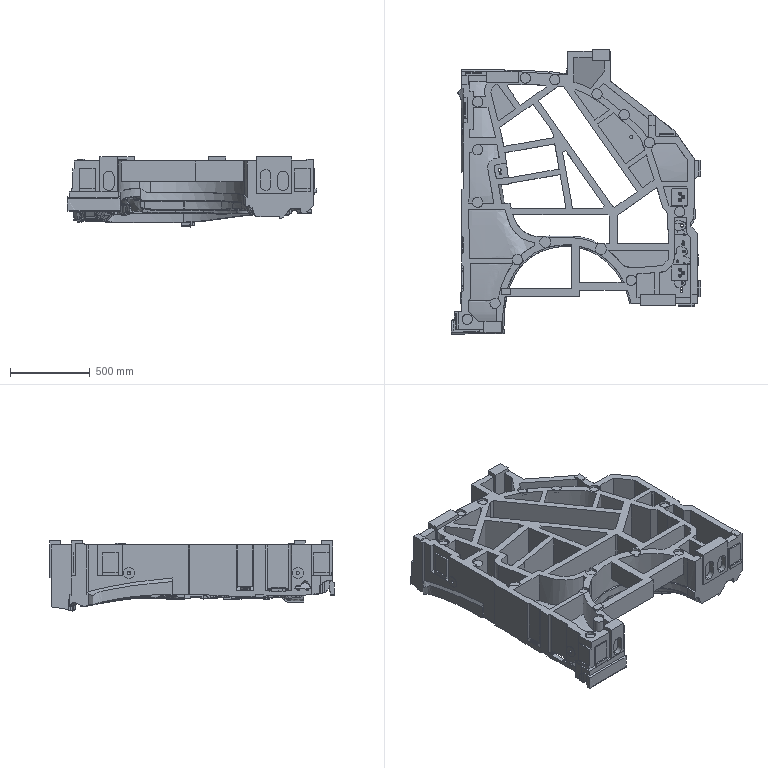Part | NX | features solid 2 | 2 solids | 2620 faces | box 1564 x 1787 x 440.073 mm | volume 250839905 mm3 | spline 1554 | plane 625 | cylinder 414 | cone 10 | torus 9 | sphere 8 | commonest cylinder face diameters 10 x60 20 x42 40 x33 65 x27 6 x25 14 x25